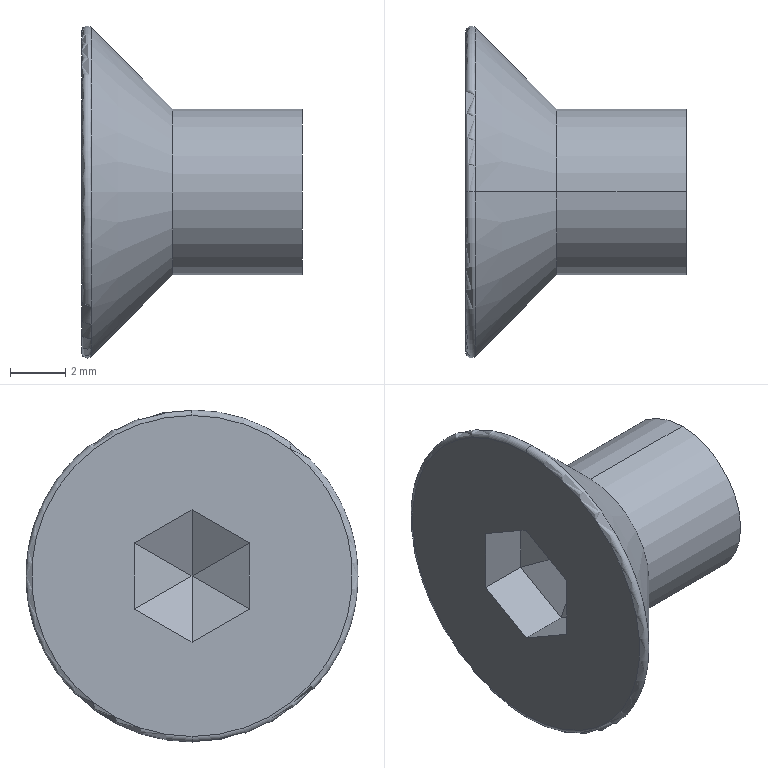Part | SolidWorks | features Cut 3, Boss 1, Extrusion 1, Fillet 1, LPattern 1, RevCut 1 | 1 solid | 20 faces | box 8 x 12.034 x 12.034 mm | volume 331.77 mm3 | plane 14 | torus 2 | cone 2 | cylinder 2 | commonest cylinder face diameters 6 x2
STEP:
#1=CARTESIAN_POINT('',(0.,0.,5.817));
#2=VERTEX_POINT('',#1);
#3=CARTESIAN_POINT('',(0.,0.,-5.817));
#4=VERTEX_POINT('',#3);
#5=CARTESIAN_POINT('',(0.,0.,0.));
#6=DIRECTION('',(-1.,0.,0.));
#7=DIRECTION('',(0.,0.,-1.));
#8=AXIS2_PLACEMENT_3D('',#5,#6,#7);
#9=CIRCLE('',#8,5.817);
#10=EDGE_CURVE('',#2,#4,#9,.T.);
#11=ORIENTED_EDGE('',*,*,#10,.F.);
#12=CARTESIAN_POINT('',(0.3414,0.,5.959));
#13=VERTEX_POINT('',#12);
#14=CARTESIAN_POINT('',(0.2,0.,5.817));
#15=DIRECTION('',(0.,1.,0.));
#16=DIRECTION('',(0.,0.,1.));
#17=AXIS2_PLACEMENT_3D('',#14,#15,#16);
#18=CIRCLE('',#17,0.2);
#19=EDGE_CURVE('',#2,#13,#18,.T.);
#20=ORIENTED_EDGE('',*,*,#19,.T.);
#21=CARTESIAN_POINT('',(0.3414,0.,-5.959));
#22=VERTEX_POINT('',#21);
#23=CARTESIAN_POINT('',(0.3414,0.,0.));
#24=DIRECTION('',(1.,0.,0.));
#25=DIRECTION('',(0.,0.,1.));
#26=AXIS2_PLACEMENT_3D('',#23,#24,#25);
#27=CIRCLE('',#26,5.959);
#28=EDGE_CURVE('',#22,#13,#27,.T.);
#29=ORIENTED_EDGE('',*,*,#28,.F.);
#30=CARTESIAN_POINT('',(0.2,0.,-5.817));
#31=DIRECTION('',(0.,-1.,0.));
#32=DIRECTION('',(0.,0.,-1.));
#33=AXIS2_PLACEMENT_3D('',#30,#31,#32);
#34=CIRCLE('',#33,0.2);
#35=EDGE_CURVE('',#4,#22,#34,.T.);
#36=ORIENTED_EDGE('',*,*,#35,.F.);
#37=EDGE_LOOP('',(#11,#20,#29,#36));
#38=FACE_OUTER_BOUND('',#37,.T.);
#39=CARTESIAN_POINT('',(0.2,0.,0.));
#40=DIRECTION('',(1.,0.,0.));
#41=DIRECTION('',(0.,0.,-1.));
#42=AXIS2_PLACEMENT_3D('',#39,#40,#41);
#43=TOROIDAL_SURFACE('',#42,5.817,0.2);
#44=ADVANCED_FACE('',(#38),#43,.T.);
#45=CARTESIAN_POINT('',(3.3,0.,3.));
#46=VERTEX_POINT('',#45);
#47=CARTESIAN_POINT('',(3.3,0.,-3.));
#48=VERTEX_POINT('',#47);
#49=CARTESIAN_POINT('',(3.3,0.,0.));
#50=DIRECTION('',(1.,0.,0.));
#51=DIRECTION('',(0.,0.,-1.));
#52=AXIS2_PLACEMENT_3D('',#49,#50,#51);
#53=CIRCLE('',#52,3.);
#54=EDGE_CURVE('',#46,#48,#53,.T.);
#55=ORIENTED_EDGE('',*,*,#54,.F.);
#56=CARTESIAN_POINT('',(3.3,0.,3.));
#57=DIRECTION('',(-0.7071,0.,0.7071));
#58=VECTOR('',#57,1000.);
#59=LINE('',#56,#58);
#60=EDGE_CURVE('',#46,#13,#59,.T.);
#61=ORIENTED_EDGE('',*,*,#60,.T.);
#62=CARTESIAN_POINT('',(0.3414,0.,0.));
#63=DIRECTION('',(1.,0.,0.));
#64=DIRECTION('',(0.,0.,1.));
#65=AXIS2_PLACEMENT_3D('',#62,#63,#64);
#66=CIRCLE('',#65,5.959);
#67=EDGE_CURVE('',#13,#22,#66,.T.);
#68=ORIENTED_EDGE('',*,*,#67,.T.);
#69=CARTESIAN_POINT('',(3.3,0.,-3.));
#70=DIRECTION('',(-0.7071,0.,-0.7071));
#71=VECTOR('',#70,1000.);
#72=LINE('',#69,#71);
#73=EDGE_CURVE('',#48,#22,#72,.T.);
#74=ORIENTED_EDGE('',*,*,#73,.F.);
#75=EDGE_LOOP('',(#55,#61,#68,#74));
#76=FACE_OUTER_BOUND('',#75,.T.);
#77=CARTESIAN_POINT('',(3.3,0.,0.));
#78=DIRECTION('',(-1.,0.,0.));
#79=DIRECTION('',(0.,0.,-1.));
#80=AXIS2_PLACEMENT_3D('',#77,#78,#79);
#81=CONICAL_SURFACE('',#80,3.,0.7854);
#82=ADVANCED_FACE('',(#76),#81,.T.);
#83=CARTESIAN_POINT('',(8.,0.,-3.));
#84=VERTEX_POINT('',#83);
#85=CARTESIAN_POINT('',(8.,0.,3.));
#86=VERTEX_POINT('',#85);
#87=CARTESIAN_POINT('',(8.,0.,0.));
#88=DIRECTION('',(1.,0.,0.));
#89=DIRECTION('',(0.,1.,0.));
#90=AXIS2_PLACEMENT_3D('',#87,#88,#89);
#91=CIRCLE('',#90,3.);
#92=EDGE_CURVE('',#84,#86,#91,.T.);
#93=ORIENTED_EDGE('',*,*,#92,.F.);
#94=CARTESIAN_POINT('',(11.3,0.,-3.));
#95=DIRECTION('',(-1.,0.,0.));
#96=VECTOR('',#95,1000.);
#97=LINE('',#94,#96);
#98=EDGE_CURVE('',#84,#48,#97,.T.);
#99=ORIENTED_EDGE('',*,*,#98,.T.);
#100=CARTESIAN_POINT('',(3.3,0.,0.));
#101=DIRECTION('',(1.,0.,0.));
#102=DIRECTION('',(0.,0.,-1.));
#103=AXIS2_PLACEMENT_3D('',#100,#101,#102);
#104=CIRCLE('',#103,3.);
#105=EDGE_CURVE('',#48,#46,#104,.T.);
#106=ORIENTED_EDGE('',*,*,#105,.T.);
#107=CARTESIAN_POINT('',(11.3,0.,3.));
#108=DIRECTION('',(-1.,0.,0.));
#109=VECTOR('',#108,1000.);
#110=LINE('',#107,#109);
#111=EDGE_CURVE('',#86,#46,#110,.T.);
#112=ORIENTED_EDGE('',*,*,#111,.F.);
#113=EDGE_LOOP('',(#93,#99,#106,#112));
#114=FACE_OUTER_BOUND('',#113,.T.);
#115=CARTESIAN_POINT('',(11.3,0.,0.));
#116=DIRECTION('',(-1.,0.,0.));
#117=DIRECTION('',(0.,0.,1.));
#118=AXIS2_PLACEMENT_3D('',#115,#116,#117);
#119=CYLINDRICAL_SURFACE('',#118,3.);
#120=ADVANCED_FACE('',(#114),#119,.T.);
#121=CARTESIAN_POINT('',(0.,0.,0.));
#122=DIRECTION('',(-1.,0.,0.));
#123=DIRECTION('',(0.,0.,-1.));
#124=AXIS2_PLACEMENT_3D('',#121,#122,#123);
#125=CIRCLE('',#124,5.817);
#126=EDGE_CURVE('',#4,#2,#125,.T.);
#127=ORIENTED_EDGE('',*,*,#126,.T.);
#128=ORIENTED_EDGE('',*,*,#10,.T.);
#129=EDGE_LOOP('',(#127,#128));
#130=FACE_OUTER_BOUND('',#129,.T.);
#131=CARTESIAN_POINT('',(0.,-2.075,-1.198));
#132=VERTEX_POINT('',#131);
#133=CARTESIAN_POINT('',(0.,0.,-2.396));
#134=VERTEX_POINT('',#133);
#135=CARTESIAN_POINT('',(0.,-2.075,-1.198));
#136=DIRECTION('',(0.,0.866,-0.5));
#137=VECTOR('',#136,1000.);
#138=LINE('',#135,#137);
#139=EDGE_CURVE('',#132,#134,#138,.T.);
#140=ORIENTED_EDGE('',*,*,#139,.T.);
#141=CARTESIAN_POINT('',(0.,2.075,-1.198));
#142=VERTEX_POINT('',#141);
#143=CARTESIAN_POINT('',(0.,0.,-2.396));
#144=DIRECTION('',(0.,0.866,0.5));
#145=VECTOR('',#144,1000.);
#146=LINE('',#143,#145);
#147=EDGE_CURVE('',#134,#142,#146,.T.);
#148=ORIENTED_EDGE('',*,*,#147,.T.);
#149=CARTESIAN_POINT('',(0.,2.075,1.198));
#150=VERTEX_POINT('',#149);
#151=CARTESIAN_POINT('',(0.,2.075,-1.198));
#152=DIRECTION('',(0.,0.,1.));
#153=VECTOR('',#152,1000.);
#154=LINE('',#151,#153);
#155=EDGE_CURVE('',#142,#150,#154,.T.);
#156=ORIENTED_EDGE('',*,*,#155,.T.);
#157=CARTESIAN_POINT('',(0.,0.,2.396));
#158=VERTEX_POINT('',#157);
#159=CARTESIAN_POINT('',(0.,2.075,1.198));
#160=DIRECTION('',(0.,-0.866,0.5));
#161=VECTOR('',#160,1000.);
#162=LINE('',#159,#161);
#163=EDGE_CURVE('',#150,#158,#162,.T.);
#164=ORIENTED_EDGE('',*,*,#163,.T.);
#165=CARTESIAN_POINT('',(0.,-2.075,1.198));
#166=VERTEX_POINT('',#165);
#167=CARTESIAN_POINT('',(0.,0.,2.396));
#168=DIRECTION('',(0.,-0.866,-0.5));
#169=VECTOR('',#168,1000.);
#170=LINE('',#167,#169);
#171=EDGE_CURVE('',#158,#166,#170,.T.);
#172=ORIENTED_EDGE('',*,*,#171,.T.);
#173=CARTESIAN_POINT('',(0.,-2.075,1.198));
#174=DIRECTION('',(0.,0.,-1.));
#175=VECTOR('',#174,1000.);
#176=LINE('',#173,#175);
#177=EDGE_CURVE('',#166,#132,#176,.T.);
#178=ORIENTED_EDGE('',*,*,#177,.T.);
#179=EDGE_LOOP('',(#140,#148,#156,#164,#172,#178));
#180=FACE_BOUND('',#179,.T.);
#181=CARTESIAN_POINT('',(0.,0.,0.));
#182=DIRECTION('',(1.,0.,0.));
#183=DIRECTION('',(0.,0.,-1.));
#184=AXIS2_PLACEMENT_3D('',#181,#182,#183);
#185=PLANE('',#184);
#186=ADVANCED_FACE('',(#130,#180),#185,.F.);
#187=ORIENTED_EDGE('',*,*,#98,.F.);
#188=CARTESIAN_POINT('',(8.,0.,0.));
#189=DIRECTION('',(1.,0.,0.));
#190=DIRECTION('',(0.,1.,0.));
#191=AXIS2_PLACEMENT_3D('',#188,#189,#190);
#192=CIRCLE('',#191,3.);
#193=EDGE_CURVE('',#86,#84,#192,.T.);
#194=ORIENTED_EDGE('',*,*,#193,.F.);
#195=ORIENTED_EDGE('',*,*,#111,.T.);
#196=ORIENTED_EDGE('',*,*,#54,.T.);
#197=EDGE_LOOP('',(#187,#194,#195,#196));
#198=FACE_OUTER_BOUND('',#197,.T.);
#199=CARTESIAN_POINT('',(11.3,0.,0.));
#200=DIRECTION('',(-1.,0.,0.));
#201=DIRECTION('',(0.,0.,1.));
#202=AXIS2_PLACEMENT_3D('',#199,#200,#201);
#203=CYLINDRICAL_SURFACE('',#202,3.);
#204=ADVANCED_FACE('',(#198),#203,.T.);
#205=ORIENTED_EDGE('',*,*,#60,.F.);
#206=ORIENTED_EDGE('',*,*,#105,.F.);
#207=ORIENTED_EDGE('',*,*,#73,.T.);
#208=ORIENTED_EDGE('',*,*,#28,.T.);
#209=EDGE_LOOP('',(#205,#206,#207,#208));
#210=FACE_OUTER_BOUND('',#209,.T.);
#211=CARTESIAN_POINT('',(3.3,0.,0.));
#212=DIRECTION('',(-1.,0.,0.));
#213=DIRECTION('',(0.,0.,-1.));
#214=AXIS2_PLACEMENT_3D('',#211,#212,#213);
#215=CONICAL_SURFACE('',#214,3.,0.7854);
#216=ADVANCED_FACE('',(#210),#215,.T.);
#217=ORIENTED_EDGE('',*,*,#193,.T.);
#218=ORIENTED_EDGE('',*,*,#92,.T.);
#219=EDGE_LOOP('',(#217,#218));
#220=FACE_OUTER_BOUND('',#219,.T.);
#221=CARTESIAN_POINT('',(8.,6.,34.25));
#222=DIRECTION('',(1.,0.,0.));
#223=DIRECTION('',(0.,1.,0.));
#224=AXIS2_PLACEMENT_3D('',#221,#222,#223);
#225=PLANE('',#224);
#226=ADVANCED_FACE('',(#220),#225,.T.);
#227=ORIENTED_EDGE('',*,*,#139,.F.);
#228=CARTESIAN_POINT('',(1.8,-2.075,-1.198));
#229=VERTEX_POINT('',#228);
#230=CARTESIAN_POINT('',(1.8,-2.075,-1.198));
#231=DIRECTION('',(-1.,0.,0.));
#232=VECTOR('',#231,1000.);
#233=LINE('',#230,#232);
#234=EDGE_CURVE('',#229,#132,#233,.T.);
#235=ORIENTED_EDGE('',*,*,#234,.F.);
#236=CARTESIAN_POINT('',(1.8,0.,-2.396));
#237=VERTEX_POINT('',#236);
#238=CARTESIAN_POINT('',(1.8,-2.075,-1.198));
#239=DIRECTION('',(0.,0.866,-0.5));
#240=VECTOR('',#239,1000.);
#241=LINE('',#238,#240);
#242=EDGE_CURVE('',#229,#237,#241,.T.);
#243=ORIENTED_EDGE('',*,*,#242,.T.);
#244=CARTESIAN_POINT('',(1.8,0.,-2.396));
#245=DIRECTION('',(-1.,0.,0.));
#246=VECTOR('',#245,1000.);
#247=LINE('',#244,#246);
#248=EDGE_CURVE('',#237,#134,#247,.T.);
#249=ORIENTED_EDGE('',*,*,#248,.T.);
#250=EDGE_LOOP('',(#227,#235,#243,#249));
#251=FACE_OUTER_BOUND('',#250,.T.);
#252=CARTESIAN_POINT('',(1.8,-2.075,-1.198));
#253=DIRECTION('',(0.,0.5,0.866));
#254=DIRECTION('',(0.,-0.866,0.5));
#255=AXIS2_PLACEMENT_3D('',#252,#253,#254);
#256=PLANE('',#255);
#257=ADVANCED_FACE('',(#251),#256,.T.);
#258=ORIENTED_EDGE('',*,*,#147,.F.);
#259=ORIENTED_EDGE('',*,*,#248,.F.);
#260=CARTESIAN_POINT('',(1.8,2.075,-1.198));
#261=VERTEX_POINT('',#260);
#262=CARTESIAN_POINT('',(1.8,0.,-2.396));
#263=DIRECTION('',(0.,0.866,0.5));
#264=VECTOR('',#263,1000.);
#265=LINE('',#262,#264);
#266=EDGE_CURVE('',#237,#261,#265,.T.);
#267=ORIENTED_EDGE('',*,*,#266,.T.);
#268=CARTESIAN_POINT('',(1.8,2.075,-1.198));
#269=DIRECTION('',(-1.,0.,0.));
#270=VECTOR('',#269,1000.);
#271=LINE('',#268,#270);
#272=EDGE_CURVE('',#261,#142,#271,.T.);
#273=ORIENTED_EDGE('',*,*,#272,.T.);
#274=EDGE_LOOP('',(#258,#259,#267,#273));
#275=FACE_OUTER_BOUND('',#274,.T.);
#276=CARTESIAN_POINT('',(1.8,0.,-2.396));
#277=DIRECTION('',(0.,-0.5,0.866));
#278=DIRECTION('',(0.,-0.866,-0.5));
#279=AXIS2_PLACEMENT_3D('',#276,#277,#278);
#280=PLANE('',#279);
#281=ADVANCED_FACE('',(#275),#280,.T.);
#282=ORIENTED_EDGE('',*,*,#155,.F.);
#283=ORIENTED_EDGE('',*,*,#272,.F.);
#284=CARTESIAN_POINT('',(1.8,2.075,1.198));
#285=VERTEX_POINT('',#284);
#286=CARTESIAN_POINT('',(1.8,2.075,-1.198));
#287=DIRECTION('',(0.,0.,1.));
#288=VECTOR('',#287,1000.);
#289=LINE('',#286,#288);
#290=EDGE_CURVE('',#261,#285,#289,.T.);
#291=ORIENTED_EDGE('',*,*,#290,.T.);
#292=CARTESIAN_POINT('',(1.8,2.075,1.198));
#293=DIRECTION('',(-1.,0.,0.));
#294=VECTOR('',#293,1000.);
#295=LINE('',#292,#294);
#296=EDGE_CURVE('',#285,#150,#295,.T.);
#297=ORIENTED_EDGE('',*,*,#296,.T.);
#298=EDGE_LOOP('',(#282,#283,#291,#297));
#299=FACE_OUTER_BOUND('',#298,.T.);
#300=CARTESIAN_POINT('',(1.8,2.075,-1.198));
#301=DIRECTION('',(0.,-1.,0.));
#302=DIRECTION('',(0.,0.,-1.));
#303=AXIS2_PLACEMENT_3D('',#300,#301,#302);
#304=PLANE('',#303);
#305=ADVANCED_FACE('',(#299),#304,.T.);
#306=ORIENTED_EDGE('',*,*,#163,.F.);
#307=ORIENTED_EDGE('',*,*,#296,.F.);
#308=CARTESIAN_POINT('',(1.8,0.,2.396));
#309=VERTEX_POINT('',#308);
#310=CARTESIAN_POINT('',(1.8,2.075,1.198));
#311=DIRECTION('',(0.,-0.866,0.5));
#312=VECTOR('',#311,1000.);
#313=LINE('',#310,#312);
#314=EDGE_CURVE('',#285,#309,#313,.T.);
#315=ORIENTED_EDGE('',*,*,#314,.T.);
#316=CARTESIAN_POINT('',(1.8,0.,2.396));
#317=DIRECTION('',(-1.,0.,0.));
#318=VECTOR('',#317,1000.);
#319=LINE('',#316,#318);
#320=EDGE_CURVE('',#309,#158,#319,.T.);
#321=ORIENTED_EDGE('',*,*,#320,.T.);
#322=EDGE_LOOP('',(#306,#307,#315,#321));
#323=FACE_OUTER_BOUND('',#322,.T.);
#324=CARTESIAN_POINT('',(1.8,2.075,1.198));
#325=DIRECTION('',(0.,-0.5,-0.866));
#326=DIRECTION('',(0.,0.866,-0.5));
#327=AXIS2_PLACEMENT_3D('',#324,#325,#326);
#328=PLANE('',#327);
#329=ADVANCED_FACE('',(#323),#328,.T.);
#330=ORIENTED_EDGE('',*,*,#171,.F.);
#331=ORIENTED_EDGE('',*,*,#320,.F.);
#332=CARTESIAN_POINT('',(1.8,-2.075,1.198));
#333=VERTEX_POINT('',#332);
#334=CARTESIAN_POINT('',(1.8,0.,2.396));
#335=DIRECTION('',(0.,-0.866,-0.5));
#336=VECTOR('',#335,1000.);
#337=LINE('',#334,#336);
#338=EDGE_CURVE('',#309,#333,#337,.T.);
#339=ORIENTED_EDGE('',*,*,#338,.T.);
#340=CARTESIAN_POINT('',(1.8,-2.075,1.198));
#341=DIRECTION('',(-1.,0.,0.));
#342=VECTOR('',#341,1000.);
#343=LINE('',#340,#342);
#344=EDGE_CURVE('',#333,#166,#343,.T.);
#345=ORIENTED_EDGE('',*,*,#344,.T.);
#346=EDGE_LOOP('',(#330,#331,#339,#345));
#347=FACE_OUTER_BOUND('',#346,.T.);
#348=CARTESIAN_POINT('',(1.8,0.,2.396));
#349=DIRECTION('',(0.,0.5,-0.866));
#350=DIRECTION('',(0.,0.866,0.5));
#351=AXIS2_PLACEMENT_3D('',#348,#349,#350);
#352=PLANE('',#351);
#353=ADVANCED_FACE('',(#347),#352,.T.);
#354=ORIENTED_EDGE('',*,*,#177,.F.);
#355=ORIENTED_EDGE('',*,*,#344,.F.);
#356=CARTESIAN_POINT('',(1.8,-2.075,1.198));
#357=DIRECTION('',(0.,0.,-1.));
#358=VECTOR('',#357,1000.);
#359=LINE('',#356,#358);
#360=EDGE_CURVE('',#333,#229,#359,.T.);
#361=ORIENTED_EDGE('',*,*,#360,.T.);
#362=ORIENTED_EDGE('',*,*,#234,.T.);
#363=EDGE_LOOP('',(#354,#355,#361,#362));
#364=FACE_OUTER_BOUND('',#363,.T.);
#365=CARTESIAN_POINT('',(1.8,-2.075,1.198));
#366=DIRECTION('',(0.,1.,0.));
#367=DIRECTION('',(0.,0.,1.));
#368=AXIS2_PLACEMENT_3D('',#365,#366,#367);
#369=PLANE('',#368);
#370=ADVANCED_FACE('',(#364),#369,.T.);
#371=ORIENTED_EDGE('',*,*,#266,.F.);
#372=CARTESIAN_POINT('',(2.998,0.,0.));
#373=VERTEX_POINT('',#372);
#374=CARTESIAN_POINT('',(1.8,0.,-2.396));
#375=DIRECTION('',(-0.4472,0.,-0.8944));
#376=VECTOR('',#375,1000.);
#377=LINE('',#374,#376);
#378=EDGE_CURVE('',#373,#237,#377,.T.);
#379=ORIENTED_EDGE('',*,*,#378,.F.);
#380=CARTESIAN_POINT('',(1.8,2.075,-1.198));
#381=DIRECTION('',(-0.4472,0.7746,-0.4472));
#382=VECTOR('',#381,1000.);
#383=LINE('',#380,#382);
#384=EDGE_CURVE('',#373,#261,#383,.T.);
#385=ORIENTED_EDGE('',*,*,#384,.T.);
#386=EDGE_LOOP('',(#371,#379,#385));
#387=FACE_OUTER_BOUND('',#386,.T.);
#388=CARTESIAN_POINT('',(1.8,0.,-2.396));
#389=DIRECTION('',(0.866,0.25,-0.433));
#390=DIRECTION('',(-0.4472,0.,-0.8944));
#391=AXIS2_PLACEMENT_3D('',#388,#389,#390);
#392=PLANE('',#391);
#393=ADVANCED_FACE('',(#387),#392,.F.);
#394=ORIENTED_EDGE('',*,*,#290,.F.);
#395=ORIENTED_EDGE('',*,*,#384,.F.);
#396=CARTESIAN_POINT('',(1.8,2.075,1.198));
#397=DIRECTION('',(-0.4472,0.7746,0.4472));
#398=VECTOR('',#397,1000.);
#399=LINE('',#396,#398);
#400=EDGE_CURVE('',#373,#285,#399,.T.);
#401=ORIENTED_EDGE('',*,*,#400,.T.);
#402=EDGE_LOOP('',(#394,#395,#401));
#403=FACE_OUTER_BOUND('',#402,.T.);
#404=CARTESIAN_POINT('',(1.8,2.075,-1.198));
#405=DIRECTION('',(0.866,0.5,0.));
#406=DIRECTION('',(-0.5,0.866,0.));
#407=AXIS2_PLACEMENT_3D('',#404,#405,#406);
#408=PLANE('',#407);
#409=ADVANCED_FACE('',(#403),#408,.F.);
#410=ORIENTED_EDGE('',*,*,#314,.F.);
#411=ORIENTED_EDGE('',*,*,#400,.F.);
#412=CARTESIAN_POINT('',(1.8,0.,2.396));
#413=DIRECTION('',(-0.4472,0.,0.8944));
#414=VECTOR('',#413,1000.);
#415=LINE('',#412,#414);
#416=EDGE_CURVE('',#373,#309,#415,.T.);
#417=ORIENTED_EDGE('',*,*,#416,.T.);
#418=EDGE_LOOP('',(#410,#411,#417));
#419=FACE_OUTER_BOUND('',#418,.T.);
#420=CARTESIAN_POINT('',(1.8,2.075,1.198));
#421=DIRECTION('',(0.866,0.25,0.433));
#422=DIRECTION('',(0.4472,0.,-0.8944));
#423=AXIS2_PLACEMENT_3D('',#420,#421,#422);
#424=PLANE('',#423);
#425=ADVANCED_FACE('',(#419),#424,.F.);
#426=ORIENTED_EDGE('',*,*,#338,.F.);
#427=ORIENTED_EDGE('',*,*,#416,.F.);
#428=CARTESIAN_POINT('',(1.8,-2.075,1.198));
#429=DIRECTION('',(-0.4472,-0.7746,0.4472));
#430=VECTOR('',#429,1000.);
#431=LINE('',#428,#430);
#432=EDGE_CURVE('',#373,#333,#431,.T.);
#433=ORIENTED_EDGE('',*,*,#432,.T.);
#434=EDGE_LOOP('',(#426,#427,#433));
#435=FACE_OUTER_BOUND('',#434,.T.);
#436=CARTESIAN_POINT('',(1.8,0.,2.396));
#437=DIRECTION('',(0.866,-0.25,0.433));
#438=DIRECTION('',(0.4472,0.,-0.8944));
#439=AXIS2_PLACEMENT_3D('',#436,#437,#438);
#440=PLANE('',#439);
#441=ADVANCED_FACE('',(#435),#440,.F.);
#442=ORIENTED_EDGE('',*,*,#360,.F.);
#443=ORIENTED_EDGE('',*,*,#432,.F.);
#444=CARTESIAN_POINT('',(1.8,-2.075,-1.198));
#445=DIRECTION('',(-0.4472,-0.7746,-0.4472));
#446=VECTOR('',#445,1000.);
#447=LINE('',#444,#446);
#448=EDGE_CURVE('',#373,#229,#447,.T.);
#449=ORIENTED_EDGE('',*,*,#448,.T.);
#450=EDGE_LOOP('',(#442,#443,#449));
#451=FACE_OUTER_BOUND('',#450,.T.);
#452=CARTESIAN_POINT('',(1.8,-2.075,1.198));
#453=DIRECTION('',(0.866,-0.5,0.));
#454=DIRECTION('',(0.5,0.866,0.));
#455=AXIS2_PLACEMENT_3D('',#452,#453,#454);
#456=PLANE('',#455);
#457=ADVANCED_FACE('',(#451),#456,.F.);
#458=ORIENTED_EDGE('',*,*,#242,.F.);
#459=ORIENTED_EDGE('',*,*,#448,.F.);
#460=ORIENTED_EDGE('',*,*,#378,.T.);
#461=EDGE_LOOP('',(#458,#459,#460));
#462=FACE_OUTER_BOUND('',#461,.T.);
#463=CARTESIAN_POINT('',(1.8,-2.075,-1.198));
#464=DIRECTION('',(0.866,-0.25,-0.433));
#465=DIRECTION('',(-0.4472,0.,-0.8944));
#466=AXIS2_PLACEMENT_3D('',#463,#464,#465);
#467=PLANE('',#466);
#468=ADVANCED_FACE('',(#462),#467,.F.);
#469=ORIENTED_EDGE('',*,*,#19,.F.);
#470=ORIENTED_EDGE('',*,*,#126,.F.);
#471=ORIENTED_EDGE('',*,*,#35,.T.);
#472=ORIENTED_EDGE('',*,*,#67,.F.);
#473=EDGE_LOOP('',(#469,#470,#471,#472));
#474=FACE_OUTER_BOUND('',#473,.T.);
#475=CARTESIAN_POINT('',(0.2,0.,0.));
#476=DIRECTION('',(1.,0.,0.));
#477=DIRECTION('',(0.,0.,-1.));
#478=AXIS2_PLACEMENT_3D('',#475,#476,#477);
#479=TOROIDAL_SURFACE('',#478,5.817,0.2);
#480=ADVANCED_FACE('',(#474),#479,.T.);
#481=CLOSED_SHELL('',(#44,#82,#120,#186,#204,#216,#226,#257,#281,#305,#329,#353,#370,#393,#409,#425,#441,#457,#468,#480));
#482=MANIFOLD_SOLID_BREP('',#481);
#483=CARTESIAN_POINT('',(0.,0.,0.));
#484=DIRECTION('',(0.,0.,1.));
#485=DIRECTION('',(1.,0.,0.));
#486=AXIS2_PLACEMENT_3D('',#483,#484,#485);
#487=(LENGTH_UNIT()NAMED_UNIT(*)SI_UNIT(.MILLI.,.METRE.));
#488=UNCERTAINTY_MEASURE_WITH_UNIT(LENGTH_MEASURE(0.00001),#487,'','');
#489=(NAMED_UNIT(*)PLANE_ANGLE_UNIT()SI_UNIT($,.RADIAN.));
#490=(NAMED_UNIT(*)SI_UNIT($,.STERADIAN.)SOLID_ANGLE_UNIT());
#491=(GEOMETRIC_REPRESENTATION_CONTEXT(3)GLOBAL_UNCERTAINTY_ASSIGNED_CONTEXT((#488))GLOBAL_UNIT_ASSIGNED_CONTEXT((#487,#489,#490))REPRESENTATION_CONTEXT('',''));
#492=ADVANCED_BREP_SHAPE_REPRESENTATION('',(#482,#486),#491);